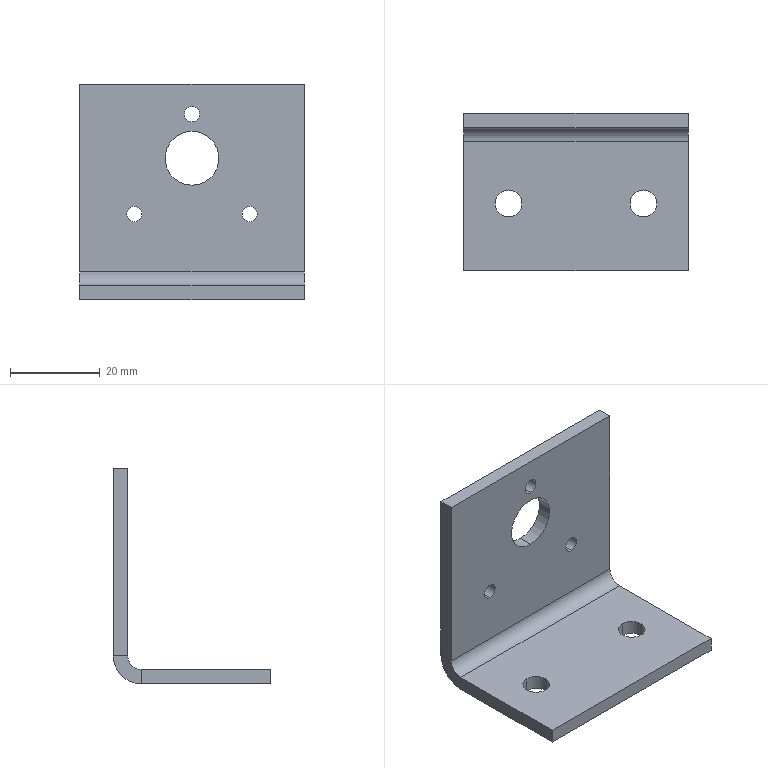Part | STEP file | 203H124123 Signal Tower BKT_Default | 1 solid | 26 faces | box 50 x 35 x 48 mm | volume 11822 mm3 | cylinder 14 | plane 12 | commonest cylinder face diameters 3.4 x6 6 x5 12 x2 12.4 x1